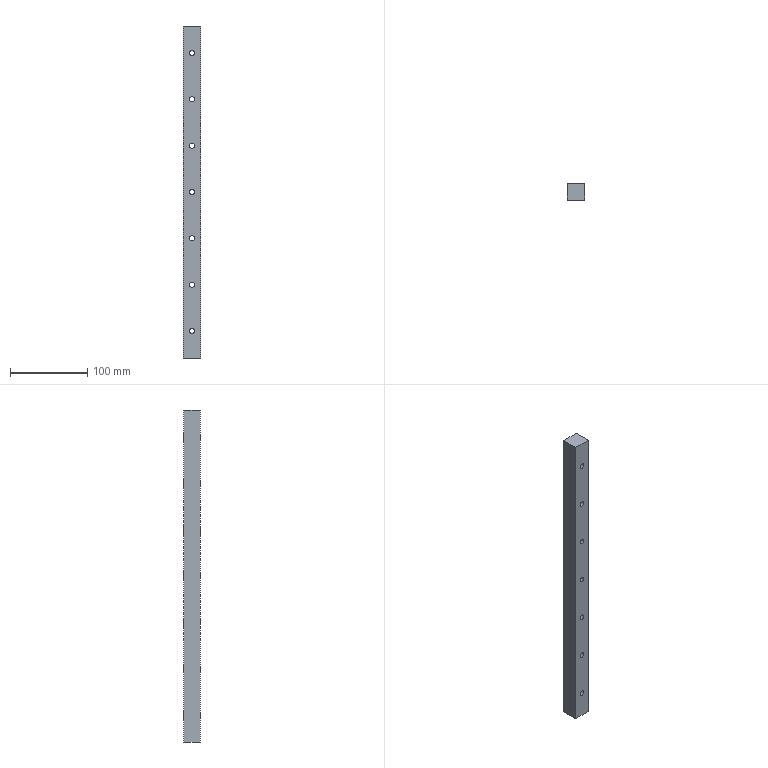Part | SolidWorks | features Extrusion 1, HoleWzd 1, LPattern 1 | 1 solid | 41 faces | box 23 x 22 x 430 mm | volume 209587 mm3 | cylinder 28 | plane 13 | commonest cylinder face diameters 6.6 x14 11 x14
STEP:
#1=CARTESIAN_POINT('',(11.5,0.,31.7));
#2=VERTEX_POINT('',#1);
#3=CARTESIAN_POINT('',(11.5,0.,38.3));
#4=VERTEX_POINT('',#3);
#5=CARTESIAN_POINT('',(11.5,0.,35.));
#6=DIRECTION('',(0.,1.,0.));
#7=DIRECTION('',(0.,0.,1.));
#8=AXIS2_PLACEMENT_3D('',#5,#6,#7);
#9=CIRCLE('',#8,3.3);
#10=EDGE_CURVE('',#2,#4,#9,.T.);
#11=ORIENTED_EDGE('',*,*,#10,.F.);
#12=CARTESIAN_POINT('',(11.5,15.6,31.7));
#13=VERTEX_POINT('',#12);
#14=CARTESIAN_POINT('',(11.5,22.,31.7));
#15=DIRECTION('',(0.,1.,0.));
#16=VECTOR('',#15,1000.);
#17=LINE('',#14,#16);
#18=EDGE_CURVE('',#2,#13,#17,.T.);
#19=ORIENTED_EDGE('',*,*,#18,.T.);
#20=CARTESIAN_POINT('',(11.5,15.6,38.3));
#21=VERTEX_POINT('',#20);
#22=CARTESIAN_POINT('',(11.5,15.6,35.));
#23=DIRECTION('',(0.,1.,0.));
#24=DIRECTION('',(0.,0.,1.));
#25=AXIS2_PLACEMENT_3D('',#22,#23,#24);
#26=CIRCLE('',#25,3.3);
#27=EDGE_CURVE('',#13,#21,#26,.T.);
#28=ORIENTED_EDGE('',*,*,#27,.T.);
#29=CARTESIAN_POINT('',(11.5,22.,38.3));
#30=DIRECTION('',(0.,1.,0.));
#31=VECTOR('',#30,1000.);
#32=LINE('',#29,#31);
#33=EDGE_CURVE('',#4,#21,#32,.T.);
#34=ORIENTED_EDGE('',*,*,#33,.F.);
#35=EDGE_LOOP('',(#11,#19,#28,#34));
#36=FACE_OUTER_BOUND('',#35,.T.);
#37=CARTESIAN_POINT('',(11.5,22.,35.));
#38=DIRECTION('',(0.,1.,0.));
#39=DIRECTION('',(0.,0.,1.));
#40=AXIS2_PLACEMENT_3D('',#37,#38,#39);
#41=CYLINDRICAL_SURFACE('',#40,3.3);
#42=ADVANCED_FACE('',(#36),#41,.F.);
#43=CARTESIAN_POINT('',(11.5,15.6,29.5));
#44=VERTEX_POINT('',#43);
#45=CARTESIAN_POINT('',(11.5,15.6,40.5));
#46=VERTEX_POINT('',#45);
#47=CARTESIAN_POINT('',(11.5,15.6,35.));
#48=DIRECTION('',(0.,1.,0.));
#49=DIRECTION('',(0.,0.,1.));
#50=AXIS2_PLACEMENT_3D('',#47,#48,#49);
#51=CIRCLE('',#50,5.5);
#52=EDGE_CURVE('',#44,#46,#51,.T.);
#53=ORIENTED_EDGE('',*,*,#52,.F.);
#54=CARTESIAN_POINT('',(11.5,22.,29.5));
#55=VERTEX_POINT('',#54);
#56=CARTESIAN_POINT('',(11.5,22.,29.5));
#57=DIRECTION('',(0.,1.,0.));
#58=VECTOR('',#57,1000.);
#59=LINE('',#56,#58);
#60=EDGE_CURVE('',#44,#55,#59,.T.);
#61=ORIENTED_EDGE('',*,*,#60,.T.);
#62=CARTESIAN_POINT('',(11.5,22.,40.5));
#63=VERTEX_POINT('',#62);
#64=CARTESIAN_POINT('',(11.5,22.,35.));
#65=DIRECTION('',(0.,1.,0.));
#66=DIRECTION('',(0.,0.,1.));
#67=AXIS2_PLACEMENT_3D('',#64,#65,#66);
#68=CIRCLE('',#67,5.5);
#69=EDGE_CURVE('',#55,#63,#68,.T.);
#70=ORIENTED_EDGE('',*,*,#69,.T.);
#71=CARTESIAN_POINT('',(11.5,22.,40.5));
#72=DIRECTION('',(0.,1.,0.));
#73=VECTOR('',#72,1000.);
#74=LINE('',#71,#73);
#75=EDGE_CURVE('',#46,#63,#74,.T.);
#76=ORIENTED_EDGE('',*,*,#75,.F.);
#77=EDGE_LOOP('',(#53,#61,#70,#76));
#78=FACE_OUTER_BOUND('',#77,.T.);
#79=CARTESIAN_POINT('',(11.5,22.,35.));
#80=DIRECTION('',(0.,1.,0.));
#81=DIRECTION('',(0.,0.,1.));
#82=AXIS2_PLACEMENT_3D('',#79,#80,#81);
#83=CYLINDRICAL_SURFACE('',#82,5.5);
#84=ADVANCED_FACE('',(#78),#83,.F.);
#85=CARTESIAN_POINT('',(11.5,0.,91.7));
#86=VERTEX_POINT('',#85);
#87=CARTESIAN_POINT('',(11.5,0.,98.3));
#88=VERTEX_POINT('',#87);
#89=CARTESIAN_POINT('',(11.5,0.,95.));
#90=DIRECTION('',(0.,1.,0.));
#91=DIRECTION('',(0.,0.,1.));
#92=AXIS2_PLACEMENT_3D('',#89,#90,#91);
#93=CIRCLE('',#92,3.3);
#94=EDGE_CURVE('',#86,#88,#93,.T.);
#95=ORIENTED_EDGE('',*,*,#94,.F.);
#96=CARTESIAN_POINT('',(11.5,15.6,91.7));
#97=VERTEX_POINT('',#96);
#98=CARTESIAN_POINT('',(11.5,22.,91.7));
#99=DIRECTION('',(0.,1.,0.));
#100=VECTOR('',#99,1000.);
#101=LINE('',#98,#100);
#102=EDGE_CURVE('',#86,#97,#101,.T.);
#103=ORIENTED_EDGE('',*,*,#102,.T.);
#104=CARTESIAN_POINT('',(11.5,15.6,98.3));
#105=VERTEX_POINT('',#104);
#106=CARTESIAN_POINT('',(11.5,15.6,95.));
#107=DIRECTION('',(0.,1.,0.));
#108=DIRECTION('',(0.,0.,1.));
#109=AXIS2_PLACEMENT_3D('',#106,#107,#108);
#110=CIRCLE('',#109,3.3);
#111=EDGE_CURVE('',#97,#105,#110,.T.);
#112=ORIENTED_EDGE('',*,*,#111,.T.);
#113=CARTESIAN_POINT('',(11.5,22.,98.3));
#114=DIRECTION('',(0.,1.,0.));
#115=VECTOR('',#114,1000.);
#116=LINE('',#113,#115);
#117=EDGE_CURVE('',#88,#105,#116,.T.);
#118=ORIENTED_EDGE('',*,*,#117,.F.);
#119=EDGE_LOOP('',(#95,#103,#112,#118));
#120=FACE_OUTER_BOUND('',#119,.T.);
#121=CARTESIAN_POINT('',(11.5,22.,95.));
#122=DIRECTION('',(0.,1.,0.));
#123=DIRECTION('',(0.,0.,1.));
#124=AXIS2_PLACEMENT_3D('',#121,#122,#123);
#125=CYLINDRICAL_SURFACE('',#124,3.3);
#126=ADVANCED_FACE('',(#120),#125,.F.);
#127=CARTESIAN_POINT('',(11.5,15.6,89.5));
#128=VERTEX_POINT('',#127);
#129=CARTESIAN_POINT('',(11.5,15.6,100.5));
#130=VERTEX_POINT('',#129);
#131=CARTESIAN_POINT('',(11.5,15.6,95.));
#132=DIRECTION('',(0.,1.,0.));
#133=DIRECTION('',(0.,0.,1.));
#134=AXIS2_PLACEMENT_3D('',#131,#132,#133);
#135=CIRCLE('',#134,5.5);
#136=EDGE_CURVE('',#128,#130,#135,.T.);
#137=ORIENTED_EDGE('',*,*,#136,.F.);
#138=CARTESIAN_POINT('',(11.5,22.,89.5));
#139=VERTEX_POINT('',#138);
#140=CARTESIAN_POINT('',(11.5,22.,89.5));
#141=DIRECTION('',(0.,1.,0.));
#142=VECTOR('',#141,1000.);
#143=LINE('',#140,#142);
#144=EDGE_CURVE('',#128,#139,#143,.T.);
#145=ORIENTED_EDGE('',*,*,#144,.T.);
#146=CARTESIAN_POINT('',(11.5,22.,100.5));
#147=VERTEX_POINT('',#146);
#148=CARTESIAN_POINT('',(11.5,22.,95.));
#149=DIRECTION('',(0.,1.,0.));
#150=DIRECTION('',(0.,0.,1.));
#151=AXIS2_PLACEMENT_3D('',#148,#149,#150);
#152=CIRCLE('',#151,5.5);
#153=EDGE_CURVE('',#139,#147,#152,.T.);
#154=ORIENTED_EDGE('',*,*,#153,.T.);
#155=CARTESIAN_POINT('',(11.5,22.,100.5));
#156=DIRECTION('',(0.,1.,0.));
#157=VECTOR('',#156,1000.);
#158=LINE('',#155,#157);
#159=EDGE_CURVE('',#130,#147,#158,.T.);
#160=ORIENTED_EDGE('',*,*,#159,.F.);
#161=EDGE_LOOP('',(#137,#145,#154,#160));
#162=FACE_OUTER_BOUND('',#161,.T.);
#163=CARTESIAN_POINT('',(11.5,22.,95.));
#164=DIRECTION('',(0.,1.,0.));
#165=DIRECTION('',(0.,0.,1.));
#166=AXIS2_PLACEMENT_3D('',#163,#164,#165);
#167=CYLINDRICAL_SURFACE('',#166,5.5);
#168=ADVANCED_FACE('',(#162),#167,.F.);
#169=CARTESIAN_POINT('',(11.5,0.,151.7));
#170=VERTEX_POINT('',#169);
#171=CARTESIAN_POINT('',(11.5,0.,158.3));
#172=VERTEX_POINT('',#171);
#173=CARTESIAN_POINT('',(11.5,0.,155.));
#174=DIRECTION('',(0.,1.,0.));
#175=DIRECTION('',(0.,0.,1.));
#176=AXIS2_PLACEMENT_3D('',#173,#174,#175);
#177=CIRCLE('',#176,3.3);
#178=EDGE_CURVE('',#170,#172,#177,.T.);
#179=ORIENTED_EDGE('',*,*,#178,.F.);
#180=CARTESIAN_POINT('',(11.5,15.6,151.7));
#181=VERTEX_POINT('',#180);
#182=CARTESIAN_POINT('',(11.5,22.,151.7));
#183=DIRECTION('',(0.,1.,0.));
#184=VECTOR('',#183,1000.);
#185=LINE('',#182,#184);
#186=EDGE_CURVE('',#170,#181,#185,.T.);
#187=ORIENTED_EDGE('',*,*,#186,.T.);
#188=CARTESIAN_POINT('',(11.5,15.6,158.3));
#189=VERTEX_POINT('',#188);
#190=CARTESIAN_POINT('',(11.5,15.6,155.));
#191=DIRECTION('',(0.,1.,0.));
#192=DIRECTION('',(0.,0.,1.));
#193=AXIS2_PLACEMENT_3D('',#190,#191,#192);
#194=CIRCLE('',#193,3.3);
#195=EDGE_CURVE('',#181,#189,#194,.T.);
#196=ORIENTED_EDGE('',*,*,#195,.T.);
#197=CARTESIAN_POINT('',(11.5,22.,158.3));
#198=DIRECTION('',(0.,1.,0.));
#199=VECTOR('',#198,1000.);
#200=LINE('',#197,#199);
#201=EDGE_CURVE('',#172,#189,#200,.T.);
#202=ORIENTED_EDGE('',*,*,#201,.F.);
#203=EDGE_LOOP('',(#179,#187,#196,#202));
#204=FACE_OUTER_BOUND('',#203,.T.);
#205=CARTESIAN_POINT('',(11.5,22.,155.));
#206=DIRECTION('',(0.,1.,0.));
#207=DIRECTION('',(0.,0.,1.));
#208=AXIS2_PLACEMENT_3D('',#205,#206,#207);
#209=CYLINDRICAL_SURFACE('',#208,3.3);
#210=ADVANCED_FACE('',(#204),#209,.F.);
#211=CARTESIAN_POINT('',(11.5,15.6,149.5));
#212=VERTEX_POINT('',#211);
#213=CARTESIAN_POINT('',(11.5,15.6,160.5));
#214=VERTEX_POINT('',#213);
#215=CARTESIAN_POINT('',(11.5,15.6,155.));
#216=DIRECTION('',(0.,1.,0.));
#217=DIRECTION('',(0.,0.,1.));
#218=AXIS2_PLACEMENT_3D('',#215,#216,#217);
#219=CIRCLE('',#218,5.5);
#220=EDGE_CURVE('',#212,#214,#219,.T.);
#221=ORIENTED_EDGE('',*,*,#220,.F.);
#222=CARTESIAN_POINT('',(11.5,22.,149.5));
#223=VERTEX_POINT('',#222);
#224=CARTESIAN_POINT('',(11.5,22.,149.5));
#225=DIRECTION('',(0.,1.,0.));
#226=VECTOR('',#225,1000.);
#227=LINE('',#224,#226);
#228=EDGE_CURVE('',#212,#223,#227,.T.);
#229=ORIENTED_EDGE('',*,*,#228,.T.);
#230=CARTESIAN_POINT('',(11.5,22.,160.5));
#231=VERTEX_POINT('',#230);
#232=CARTESIAN_POINT('',(11.5,22.,155.));
#233=DIRECTION('',(0.,1.,0.));
#234=DIRECTION('',(0.,0.,1.));
#235=AXIS2_PLACEMENT_3D('',#232,#233,#234);
#236=CIRCLE('',#235,5.5);
#237=EDGE_CURVE('',#223,#231,#236,.T.);
#238=ORIENTED_EDGE('',*,*,#237,.T.);
#239=CARTESIAN_POINT('',(11.5,22.,160.5));
#240=DIRECTION('',(0.,1.,0.));
#241=VECTOR('',#240,1000.);
#242=LINE('',#239,#241);
#243=EDGE_CURVE('',#214,#231,#242,.T.);
#244=ORIENTED_EDGE('',*,*,#243,.F.);
#245=EDGE_LOOP('',(#221,#229,#238,#244));
#246=FACE_OUTER_BOUND('',#245,.T.);
#247=CARTESIAN_POINT('',(11.5,22.,155.));
#248=DIRECTION('',(0.,1.,0.));
#249=DIRECTION('',(0.,0.,1.));
#250=AXIS2_PLACEMENT_3D('',#247,#248,#249);
#251=CYLINDRICAL_SURFACE('',#250,5.5);
#252=ADVANCED_FACE('',(#246),#251,.F.);
#253=CARTESIAN_POINT('',(11.5,0.,211.7));
#254=VERTEX_POINT('',#253);
#255=CARTESIAN_POINT('',(11.5,0.,218.3));
#256=VERTEX_POINT('',#255);
#257=CARTESIAN_POINT('',(11.5,0.,215.));
#258=DIRECTION('',(0.,1.,0.));
#259=DIRECTION('',(0.,0.,1.));
#260=AXIS2_PLACEMENT_3D('',#257,#258,#259);
#261=CIRCLE('',#260,3.3);
#262=EDGE_CURVE('',#254,#256,#261,.T.);
#263=ORIENTED_EDGE('',*,*,#262,.F.);
#264=CARTESIAN_POINT('',(11.5,15.6,211.7));
#265=VERTEX_POINT('',#264);
#266=CARTESIAN_POINT('',(11.5,22.,211.7));
#267=DIRECTION('',(0.,1.,0.));
#268=VECTOR('',#267,1000.);
#269=LINE('',#266,#268);
#270=EDGE_CURVE('',#254,#265,#269,.T.);
#271=ORIENTED_EDGE('',*,*,#270,.T.);
#272=CARTESIAN_POINT('',(11.5,15.6,218.3));
#273=VERTEX_POINT('',#272);
#274=CARTESIAN_POINT('',(11.5,15.6,215.));
#275=DIRECTION('',(0.,1.,0.));
#276=DIRECTION('',(0.,0.,1.));
#277=AXIS2_PLACEMENT_3D('',#274,#275,#276);
#278=CIRCLE('',#277,3.3);
#279=EDGE_CURVE('',#265,#273,#278,.T.);
#280=ORIENTED_EDGE('',*,*,#279,.T.);
#281=CARTESIAN_POINT('',(11.5,22.,218.3));
#282=DIRECTION('',(0.,1.,0.));
#283=VECTOR('',#282,1000.);
#284=LINE('',#281,#283);
#285=EDGE_CURVE('',#256,#273,#284,.T.);
#286=ORIENTED_EDGE('',*,*,#285,.F.);
#287=EDGE_LOOP('',(#263,#271,#280,#286));
#288=FACE_OUTER_BOUND('',#287,.T.);
#289=CARTESIAN_POINT('',(11.5,22.,215.));
#290=DIRECTION('',(0.,1.,0.));
#291=DIRECTION('',(0.,0.,1.));
#292=AXIS2_PLACEMENT_3D('',#289,#290,#291);
#293=CYLINDRICAL_SURFACE('',#292,3.3);
#294=ADVANCED_FACE('',(#288),#293,.F.);
#295=CARTESIAN_POINT('',(11.5,15.6,209.5));
#296=VERTEX_POINT('',#295);
#297=CARTESIAN_POINT('',(11.5,15.6,220.5));
#298=VERTEX_POINT('',#297);
#299=CARTESIAN_POINT('',(11.5,15.6,215.));
#300=DIRECTION('',(0.,1.,0.));
#301=DIRECTION('',(0.,0.,1.));
#302=AXIS2_PLACEMENT_3D('',#299,#300,#301);
#303=CIRCLE('',#302,5.5);
#304=EDGE_CURVE('',#296,#298,#303,.T.);
#305=ORIENTED_EDGE('',*,*,#304,.F.);
#306=CARTESIAN_POINT('',(11.5,22.,209.5));
#307=VERTEX_POINT('',#306);
#308=CARTESIAN_POINT('',(11.5,22.,209.5));
#309=DIRECTION('',(0.,1.,0.));
#310=VECTOR('',#309,1000.);
#311=LINE('',#308,#310);
#312=EDGE_CURVE('',#296,#307,#311,.T.);
#313=ORIENTED_EDGE('',*,*,#312,.T.);
#314=CARTESIAN_POINT('',(11.5,22.,220.5));
#315=VERTEX_POINT('',#314);
#316=CARTESIAN_POINT('',(11.5,22.,215.));
#317=DIRECTION('',(0.,1.,0.));
#318=DIRECTION('',(0.,0.,1.));
#319=AXIS2_PLACEMENT_3D('',#316,#317,#318);
#320=CIRCLE('',#319,5.5);
#321=EDGE_CURVE('',#307,#315,#320,.T.);
#322=ORIENTED_EDGE('',*,*,#321,.T.);
#323=CARTESIAN_POINT('',(11.5,22.,220.5));
#324=DIRECTION('',(0.,1.,0.));
#325=VECTOR('',#324,1000.);
#326=LINE('',#323,#325);
#327=EDGE_CURVE('',#298,#315,#326,.T.);
#328=ORIENTED_EDGE('',*,*,#327,.F.);
#329=EDGE_LOOP('',(#305,#313,#322,#328));
#330=FACE_OUTER_BOUND('',#329,.T.);
#331=CARTESIAN_POINT('',(11.5,22.,215.));
#332=DIRECTION('',(0.,1.,0.));
#333=DIRECTION('',(0.,0.,1.));
#334=AXIS2_PLACEMENT_3D('',#331,#332,#333);
#335=CYLINDRICAL_SURFACE('',#334,5.5);
#336=ADVANCED_FACE('',(#330),#335,.F.);
#337=CARTESIAN_POINT('',(11.5,0.,271.7));
#338=VERTEX_POINT('',#337);
#339=CARTESIAN_POINT('',(11.5,0.,278.3));
#340=VERTEX_POINT('',#339);
#341=CARTESIAN_POINT('',(11.5,0.,275.));
#342=DIRECTION('',(0.,1.,0.));
#343=DIRECTION('',(0.,0.,1.));
#344=AXIS2_PLACEMENT_3D('',#341,#342,#343);
#345=CIRCLE('',#344,3.3);
#346=EDGE_CURVE('',#338,#340,#345,.T.);
#347=ORIENTED_EDGE('',*,*,#346,.F.);
#348=CARTESIAN_POINT('',(11.5,15.6,271.7));
#349=VERTEX_POINT('',#348);
#350=CARTESIAN_POINT('',(11.5,22.,271.7));
#351=DIRECTION('',(0.,1.,0.));
#352=VECTOR('',#351,1000.);
#353=LINE('',#350,#352);
#354=EDGE_CURVE('',#338,#349,#353,.T.);
#355=ORIENTED_EDGE('',*,*,#354,.T.);
#356=CARTESIAN_POINT('',(11.5,15.6,278.3));
#357=VERTEX_POINT('',#356);
#358=CARTESIAN_POINT('',(11.5,15.6,275.));
#359=DIRECTION('',(0.,1.,0.));
#360=DIRECTION('',(0.,0.,1.));
#361=AXIS2_PLACEMENT_3D('',#358,#359,#360);
#362=CIRCLE('',#361,3.3);
#363=EDGE_CURVE('',#349,#357,#362,.T.);
#364=ORIENTED_EDGE('',*,*,#363,.T.);
#365=CARTESIAN_POINT('',(11.5,22.,278.3));
#366=DIRECTION('',(0.,1.,0.));
#367=VECTOR('',#366,1000.);
#368=LINE('',#365,#367);
#369=EDGE_CURVE('',#340,#357,#368,.T.);
#370=ORIENTED_EDGE('',*,*,#369,.F.);
#371=EDGE_LOOP('',(#347,#355,#364,#370));
#372=FACE_OUTER_BOUND('',#371,.T.);
#373=CARTESIAN_POINT('',(11.5,22.,275.));
#374=DIRECTION('',(0.,1.,0.));
#375=DIRECTION('',(0.,0.,1.));
#376=AXIS2_PLACEMENT_3D('',#373,#374,#375);
#377=CYLINDRICAL_SURFACE('',#376,3.3);
#378=ADVANCED_FACE('',(#372),#377,.F.);
#379=CARTESIAN_POINT('',(11.5,15.6,269.5));
#380=VERTEX_POINT('',#379);
#381=CARTESIAN_POINT('',(11.5,15.6,280.5));
#382=VERTEX_POINT('',#381);
#383=CARTESIAN_POINT('',(11.5,15.6,275.));
#384=DIRECTION('',(0.,1.,0.));
#385=DIRECTION('',(0.,0.,1.));
#386=AXIS2_PLACEMENT_3D('',#383,#384,#385);
#387=CIRCLE('',#386,5.5);
#388=EDGE_CURVE('',#380,#382,#387,.T.);
#389=ORIENTED_EDGE('',*,*,#388,.F.);
#390=CARTESIAN_POINT('',(11.5,22.,269.5));
#391=VERTEX_POINT('',#390);
#392=CARTESIAN_POINT('',(11.5,22.,269.5));
#393=DIRECTION('',(0.,1.,0.));
#394=VECTOR('',#393,1000.);
#395=LINE('',#392,#394);
#396=EDGE_CURVE('',#380,#391,#395,.T.);
#397=ORIENTED_EDGE('',*,*,#396,.T.);
#398=CARTESIAN_POINT('',(11.5,22.,280.5));
#399=VERTEX_POINT('',#398);
#400=CARTESIAN_POINT('',(11.5,22.,275.));
#401=DIRECTION('',(0.,1.,0.));
#402=DIRECTION('',(0.,0.,1.));
#403=AXIS2_PLACEMENT_3D('',#400,#401,#402);
#404=CIRCLE('',#403,5.5);
#405=EDGE_CURVE('',#391,#399,#404,.T.);
#406=ORIENTED_EDGE('',*,*,#405,.T.);
#407=CARTESIAN_POINT('',(11.5,22.,280.5));
#408=DIRECTION('',(0.,1.,0.));
#409=VECTOR('',#408,1000.);
#410=LINE('',#407,#409);
#411=EDGE_CURVE('',#382,#399,#410,.T.);
#412=ORIENTED_EDGE('',*,*,#411,.F.);
#413=EDGE_LOOP('',(#389,#397,#406,#412));
#414=FACE_OUTER_BOUND('',#413,.T.);
#415=CARTESIAN_POINT('',(11.5,22.,275.));
#416=DIRECTION('',(0.,1.,0.));
#417=DIRECTION('',(0.,0.,1.));
#418=AXIS2_PLACEMENT_3D('',#415,#416,#417);
#419=CYLINDRICAL_SURFACE('',#418,5.5);
#420=ADVANCED_FACE('',(#414),#419,.F.);
#421=CARTESIAN_POINT('',(11.5,15.6,329.5));
#422=VERTEX_POINT('',#421);
#423=CARTESIAN_POINT('',(11.5,15.6,340.5));
#424=VERTEX_POINT('',#423);
#425=CARTESIAN_POINT('',(11.5,15.6,335.));
#426=DIRECTION('',(0.,1.,0.));
#427=DIRECTION('',(0.,0.,1.));
#428=AXIS2_PLACEMENT_3D('',#425,#426,#427);
#429=CIRCLE('',#428,5.5);
#430=EDGE_CURVE('',#422,#424,#429,.T.);
#431=ORIENTED_EDGE('',*,*,#430,.F.);
#432=CARTESIAN_POINT('',(11.5,22.,329.5));
#433=VERTEX_POINT('',#432);
#434=CARTESIAN_POINT('',(11.5,22.,329.5));
#435=DIRECTION('',(0.,1.,0.));
#436=VECTOR('',#435,1000.);
#437=LINE('',#434,#436);
#438=EDGE_CURVE('',#422,#433,#437,.T.);
#439=ORIENTED_EDGE('',*,*,#438,.T.);
#440=CARTESIAN_POINT('',(11.5,22.,340.5));
#441=VERTEX_POINT('',#440);
#442=CARTESIAN_POINT('',(11.5,22.,335.));
#443=DIRECTION('',(0.,1.,0.));
#444=DIRECTION('',(0.,0.,1.));
#445=AXIS2_PLACEMENT_3D('',#442,#443,#444);
#446=CIRCLE('',#445,5.5);
#447=EDGE_CURVE('',#433,#441,#446,.T.);
#448=ORIENTED_EDGE('',*,*,#447,.T.);
#449=CARTESIAN_POINT('',(11.5,22.,340.5));
#450=DIRECTION('',(0.,1.,0.));
#451=VECTOR('',#450,1000.);
#452=LINE('',#449,#451);
#453=EDGE_CURVE('',#424,#441,#452,.T.);
#454=ORIENTED_EDGE('',*,*,#453,.F.);
#455=EDGE_LOOP('',(#431,#439,#448,#454));
#456=FACE_OUTER_BOUND('',#455,.T.);
#457=CARTESIAN_POINT('',(11.5,22.,335.));
#458=DIRECTION('',(0.,1.,0.));
#459=DIRECTION('',(0.,0.,1.));
#460=AXIS2_PLACEMENT_3D('',#457,#458,#459);
#461=CYLINDRICAL_SURFACE('',#460,5.5);
#462=ADVANCED_FACE('',(#456),#461,.F.);
#463=CARTESIAN_POINT('',(11.5,0.,331.7));
#464=VERTEX_POINT('',#463);
#465=CARTESIAN_POINT('',(11.5,0.,338.3));
#466=VERTEX_POINT('',#465);
#467=CARTESIAN_POINT('',(11.5,0.,335.));
#468=DIRECTION('',(0.,1.,0.));
#469=DIRECTION('',(0.,0.,1.));
#470=AXIS2_PLACEMENT_3D('',#467,#468,#469);
#471=CIRCLE('',#470,3.3);
#472=EDGE_CURVE('',#464,#466,#471,.T.);
#473=ORIENTED_EDGE('',*,*,#472,.F.);
#474=CARTESIAN_POINT('',(11.5,15.6,331.7));
#475=VERTEX_POINT('',#474);
#476=CARTESIAN_POINT('',(11.5,22.,331.7));
#477=DIRECTION('',(0.,1.,0.));
#478=VECTOR('',#477,1000.);
#479=LINE('',#476,#478);
#480=EDGE_CURVE('',#464,#475,#479,.T.);
#481=ORIENTED_EDGE('',*,*,#480,.T.);
#482=CARTESIAN_POINT('',(11.5,15.6,338.3));
#483=VERTEX_POINT('',#482);
#484=CARTESIAN_POINT('',(11.5,15.6,335.));
#485=DIRECTION('',(0.,1.,0.));
#486=DIRECTION('',(0.,0.,1.));
#487=AXIS2_PLACEMENT_3D('',#484,#485,#486);
#488=CIRCLE('',#487,3.3);
#489=EDGE_CURVE('',#475,#483,#488,.T.);
#490=ORIENTED_EDGE('',*,*,#489,.T.);
#491=CARTESIAN_POINT('',(11.5,22.,338.3));
#492=DIRECTION('',(0.,1.,0.));
#493=VECTOR('',#492,1000.);
#494=LINE('',#491,#493);
#495=EDGE_CURVE('',#466,#483,#494,.T.);
#496=ORIENTED_EDGE('',*,*,#495,.F.);
#497=EDGE_LOOP('',(#473,#481,#490,#496));
#498=FACE_OUTER_BOUND('',#497,.T.);
#499=CARTESIAN_POINT('',(11.5,22.,335.));
#500=DIRECTION('',(0.,1.,0.));
#501=DIRECTION('',(0.,0.,1.));
#502=AXIS2_PLACEMENT_3D('',#499,#500,#501);
#503=CYLINDRICAL_SURFACE('',#502,3.3);
#504=ADVANCED_FACE('',(#498),#503,.F.);
#505=CARTESIAN_POINT('',(11.5,15.6,389.5));
#506=VERTEX_POINT('',#505);
#507=CARTESIAN_POINT('',(11.5,15.6,400.5));
#508=VERTEX_POINT('',#507);
#509=CARTESIAN_POINT('',(11.5,15.6,395.));
#510=DIRECTION('',(0.,1.,0.));
#511=DIRECTION('',(0.,0.,1.));
#512=AXIS2_PLACEMENT_3D('',#509,#510,#511);
#513=CIRCLE('',#512,5.5);
#514=EDGE_CURVE('',#506,#508,#513,.T.);
#515=ORIENTED_EDGE('',*,*,#514,.F.);
#516=CARTESIAN_POINT('',(11.5,22.,389.5));
#517=VERTEX_POINT('',#516);
#518=CARTESIAN_POINT('',(11.5,22.,389.5));
#519=DIRECTION('',(0.,1.,0.));
#520=VECTOR('',#519,1000.);
#521=LINE('',#518,#520);
#522=EDGE_CURVE('',#506,#517,#521,.T.);
#523=ORIENTED_EDGE('',*,*,#522,.T.);
#524=CARTESIAN_POINT('',(11.5,22.,400.5));
#525=VERTEX_POINT('',#524);
#526=CARTESIAN_POINT('',(11.5,22.,395.));
#527=DIRECTION('',(0.,1.,0.));
#528=DIRECTION('',(0.,0.,1.));
#529=AXIS2_PLACEMENT_3D('',#526,#527,#528);
#530=CIRCLE('',#529,5.5);
#531=EDGE_CURVE('',#517,#525,#530,.T.);
#532=ORIENTED_EDGE('',*,*,#531,.T.);
#533=CARTESIAN_POINT('',(11.5,22.,400.5));
#534=DIRECTION('',(0.,1.,0.));
#535=VECTOR('',#534,1000.);
#536=LINE('',#533,#535);
#537=EDGE_CURVE('',#508,#525,#536,.T.);
#538=ORIENTED_EDGE('',*,*,#537,.F.);
#539=EDGE_LOOP('',(#515,#523,#532,#538));
#540=FACE_OUTER_BOUND('',#539,.T.);
#541=CARTESIAN_POINT('',(11.5,22.,395.));
#542=DIRECTION('',(0.,1.,0.));
#543=DIRECTION('',(0.,0.,1.));
#544=AXIS2_PLACEMENT_3D('',#541,#542,#543);
#545=CYLINDRICAL_SURFACE('',#544,5.5);
#546=ADVANCED_FACE('',(#540),#545,.F.);
#547=CARTESIAN_POINT('',(11.5,0.,391.7));
#548=VERTEX_POINT('',#547);
#549=CARTESIAN_POINT('',(11.5,0.,398.3));
#550=VERTEX_POINT('',#549);
#551=CARTESIAN_POINT('',(11.5,0.,395.));
#552=DIRECTION('',(0.,1.,0.));
#553=DIRECTION('',(0.,0.,1.));
#554=AXIS2_PLACEMENT_3D('',#551,#552,#553);
#555=CIRCLE('',#554,3.3);
#556=EDGE_CURVE('',#548,#550,#555,.T.);
#557=ORIENTED_EDGE('',*,*,#556,.F.);
#558=CARTESIAN_POINT('',(11.5,15.6,391.7));
#559=VERTEX_POINT('',#558);
#560=CARTESIAN_POINT('',(11.5,22.,391.7));
#561=DIRECTION('',(0.,1.,0.));
#562=VECTOR('',#561,1000.);
#563=LINE('',#560,#562);
#564=EDGE_CURVE('',#548,#559,#563,.T.);
#565=ORIENTED_EDGE('',*,*,#564,.T.);
#566=CARTESIAN_POINT('',(11.5,15.6,398.3));
#567=VERTEX_POINT('',#566);
#568=CARTESIAN_POINT('',(11.5,15.6,395.));
#569=DIRECTION('',(0.,1.,0.));
#570=DIRECTION('',(0.,0.,1.));
#571=AXIS2_PLACEMENT_3D('',#568,#569,#570);
#572=CIRCLE('',#571,3.3);
#573=EDGE_CURVE('',#559,#567,#572,.T.);
#574=ORIENTED_EDGE('',*,*,#573,.T.);
#575=CARTESIAN_POINT('',(11.5,22.,398.3));
#576=DIRECTION('',(0.,1.,0.));
#577=VECTOR('',#576,1000.);
#578=LINE('',#575,#577);
#579=EDGE_CURVE('',#550,#567,#578,.T.);
#580=ORIENTED_EDGE('',*,*,#579,.F.);
#581=EDGE_LOOP('',(#557,#565,#574,#580));
#582=FACE_OUTER_BOUND('',#581,.T.);
#583=CARTESIAN_POINT('',(11.5,22.,395.));
#584=DIRECTION('',(0.,1.,0.));
#585=DIRECTION('',(0.,0.,1.));
#586=AXIS2_PLACEMENT_3D('',#583,#584,#585);
#587=CYLINDRICAL_SURFACE('',#586,3.3);
#588=ADVANCED_FACE('',(#582),#587,.F.);
#589=CARTESIAN_POINT('',(0.,22.,0.));
#590=VERTEX_POINT('',#589);
#591=CARTESIAN_POINT('',(0.,0.,0.));
#592=VERTEX_POINT('',#591);
#593=CARTESIAN_POINT('',(0.,0.,0.));
#594=DIRECTION('',(0.,-1.,0.));
#595=VECTOR('',#594,1000.);
#596=LINE('',#593,#595);
#597=EDGE_CURVE('',#590,#592,#596,.T.);
#598=ORIENTED_EDGE('',*,*,#597,.T.);
#599=CARTESIAN_POINT('',(0.,0.,430.));
#600=VERTEX_POINT('',#599);
#601=CARTESIAN_POINT('',(0.,0.,430.));
#602=DIRECTION('',(0.,0.,-1.));
#603=VECTOR('',#602,1000.);
#604=LINE('',#601,#603);
#605=EDGE_CURVE('',#600,#592,#604,.T.);
#606=ORIENTED_EDGE('',*,*,#605,.F.);
#607=CARTESIAN_POINT('',(0.,22.,430.));
#608=VERTEX_POINT('',#607);
#609=CARTESIAN_POINT('',(0.,0.,430.));
#610=DIRECTION('',(0.,-1.,0.));
#611=VECTOR('',#610,1000.);
#612=LINE('',#609,#611);
#613=EDGE_CURVE('',#608,#600,#612,.T.);
#614=ORIENTED_EDGE('',*,*,#613,.F.);
#615=CARTESIAN_POINT('',(0.,22.,430.));
#616=DIRECTION('',(0.,0.,-1.));
#617=VECTOR('',#616,1000.);
#618=LINE('',#615,#617);
#619=EDGE_CURVE('',#608,#590,#618,.T.);
#620=ORIENTED_EDGE('',*,*,#619,.T.);
#621=EDGE_LOOP('',(#598,#606,#614,#620));
#622=FACE_OUTER_BOUND('',#621,.T.);
#623=CARTESIAN_POINT('',(0.,0.,430.));
#624=DIRECTION('',(1.,0.,0.));
#625=DIRECTION('',(0.,1.,0.));
#626=AXIS2_PLACEMENT_3D('',#623,#624,#625);
#627=PLANE('',#626);
#628=ADVANCED_FACE('',(#622),#627,.F.);
#629=CARTESIAN_POINT('',(11.5,0.,335.));
#630=DIRECTION('',(0.,1.,0.));
#631=DIRECTION('',(0.,0.,1.));
#632=AXIS2_PLACEMENT_3D('',#629,#630,#631);
#633=CIRCLE('',#632,3.3);
#634=EDGE_CURVE('',#466,#464,#633,.T.);
#635=ORIENTED_EDGE('',*,*,#634,.T.);
#636=ORIENTED_EDGE('',*,*,#472,.T.);
#637=EDGE_LOOP('',(#635,#636));
#638=FACE_BOUND('',#637,.T.);
#639=CARTESIAN_POINT('',(11.5,0.,395.));
#640=DIRECTION('',(0.,1.,0.));
#641=DIRECTION('',(0.,0.,1.));
#642=AXIS2_PLACEMENT_3D('',#639,#640,#641);
#643=CIRCLE('',#642,3.3);
#644=EDGE_CURVE('',#550,#548,#643,.T.);
#645=ORIENTED_EDGE('',*,*,#644,.T.);
#646=ORIENTED_EDGE('',*,*,#556,.T.);
#647=EDGE_LOOP('',(#645,#646));
#648=FACE_BOUND('',#647,.T.);
#649=CARTESIAN_POINT('',(23.,0.,0.));
#650=VERTEX_POINT('',#649);
#651=CARTESIAN_POINT('',(0.,0.,0.));
#652=DIRECTION('',(1.,0.,0.));
#653=VECTOR('',#652,1000.);
#654=LINE('',#651,#653);
#655=EDGE_CURVE('',#592,#650,#654,.T.);
#656=ORIENTED_EDGE('',*,*,#655,.T.);
#657=CARTESIAN_POINT('',(23.,0.,430.));
#658=VERTEX_POINT('',#657);
#659=CARTESIAN_POINT('',(23.,0.,430.));
#660=DIRECTION('',(0.,0.,-1.));
#661=VECTOR('',#660,1000.);
#662=LINE('',#659,#661);
#663=EDGE_CURVE('',#658,#650,#662,.T.);
#664=ORIENTED_EDGE('',*,*,#663,.F.);
#665=CARTESIAN_POINT('',(0.,0.,430.));
#666=DIRECTION('',(1.,0.,0.));
#667=VECTOR('',#666,1000.);
#668=LINE('',#665,#667);
#669=EDGE_CURVE('',#600,#658,#668,.T.);
#670=ORIENTED_EDGE('',*,*,#669,.F.);
#671=ORIENTED_EDGE('',*,*,#605,.T.);
#672=EDGE_LOOP('',(#656,#664,#670,#671));
#673=FACE_OUTER_BOUND('',#672,.T.);
#674=CARTESIAN_POINT('',(11.5,0.,275.));
#675=DIRECTION('',(0.,1.,0.));
#676=DIRECTION('',(0.,0.,1.));
#677=AXIS2_PLACEMENT_3D('',#674,#675,#676);
#678=CIRCLE('',#677,3.3);
#679=EDGE_CURVE('',#340,#338,#678,.T.);
#680=ORIENTED_EDGE('',*,*,#679,.T.);
#681=ORIENTED_EDGE('',*,*,#346,.T.);
#682=EDGE_LOOP('',(#680,#681));
#683=FACE_BOUND('',#682,.T.);
#684=CARTESIAN_POINT('',(11.5,0.,215.));
#685=DIRECTION('',(0.,1.,0.));
#686=DIRECTION('',(0.,0.,1.));
#687=AXIS2_PLACEMENT_3D('',#684,#685,#686);
#688=CIRCLE('',#687,3.3);
#689=EDGE_CURVE('',#256,#254,#688,.T.);
#690=ORIENTED_EDGE('',*,*,#689,.T.);
#691=ORIENTED_EDGE('',*,*,#262,.T.);
#692=EDGE_LOOP('',(#690,#691));
#693=FACE_BOUND('',#692,.T.);
#694=CARTESIAN_POINT('',(11.5,0.,155.));
#695=DIRECTION('',(0.,1.,0.));
#696=DIRECTION('',(0.,0.,1.));
#697=AXIS2_PLACEMENT_3D('',#694,#695,#696);
#698=CIRCLE('',#697,3.3);
#699=EDGE_CURVE('',#172,#170,#698,.T.);
#700=ORIENTED_EDGE('',*,*,#699,.T.);
#701=ORIENTED_EDGE('',*,*,#178,.T.);
#702=EDGE_LOOP('',(#700,#701));
#703=FACE_BOUND('',#702,.T.);
#704=CARTESIAN_POINT('',(11.5,0.,95.));
#705=DIRECTION('',(0.,1.,0.));
#706=DIRECTION('',(0.,0.,1.));
#707=AXIS2_PLACEMENT_3D('',#704,#705,#706);
#708=CIRCLE('',#707,3.3);
#709=EDGE_CURVE('',#88,#86,#708,.T.);
#710=ORIENTED_EDGE('',*,*,#709,.T.);
#711=ORIENTED_EDGE('',*,*,#94,.T.);
#712=EDGE_LOOP('',(#710,#711));
#713=FACE_BOUND('',#712,.T.);
#714=CARTESIAN_POINT('',(11.5,0.,35.));
#715=DIRECTION('',(0.,1.,0.));
#716=DIRECTION('',(0.,0.,1.));
#717=AXIS2_PLACEMENT_3D('',#714,#715,#716);
#718=CIRCLE('',#717,3.3);
#719=EDGE_CURVE('',#4,#2,#718,.T.);
#720=ORIENTED_EDGE('',*,*,#719,.T.);
#721=ORIENTED_EDGE('',*,*,#10,.T.);
#722=EDGE_LOOP('',(#720,#721));
#723=FACE_BOUND('',#722,.T.);
#724=CARTESIAN_POINT('',(0.,0.,430.));
#725=DIRECTION('',(0.,1.,0.));
#726=DIRECTION('',(0.,0.,1.));
#727=AXIS2_PLACEMENT_3D('',#724,#725,#726);
#728=PLANE('',#727);
#729=ADVANCED_FACE('',(#638,#648,#673,#683,#693,#703,#713,#723),#728,.F.);
#730=CARTESIAN_POINT('',(23.,22.,0.));
#731=VERTEX_POINT('',#730);
#732=CARTESIAN_POINT('',(23.,0.,0.));
#733=DIRECTION('',(0.,1.,0.));
#734=VECTOR('',#733,1000.);
#735=LINE('',#732,#734);
#736=EDGE_CURVE('',#650,#731,#735,.T.);
#737=ORIENTED_EDGE('',*,*,#736,.T.);
#738=CARTESIAN_POINT('',(23.,22.,430.));
#739=VERTEX_POINT('',#738);
#740=CARTESIAN_POINT('',(23.,22.,430.));
#741=DIRECTION('',(0.,0.,-1.));
#742=VECTOR('',#741,1000.);
#743=LINE('',#740,#742);
#744=EDGE_CURVE('',#739,#731,#743,.T.);
#745=ORIENTED_EDGE('',*,*,#744,.F.);
#746=CARTESIAN_POINT('',(23.,0.,430.));
#747=DIRECTION('',(0.,1.,0.));
#748=VECTOR('',#747,1000.);
#749=LINE('',#746,#748);
#750=EDGE_CURVE('',#658,#739,#749,.T.);
#751=ORIENTED_EDGE('',*,*,#750,.F.);
#752=ORIENTED_EDGE('',*,*,#663,.T.);
#753=EDGE_LOOP('',(#737,#745,#751,#752));
#754=FACE_OUTER_BOUND('',#753,.T.);
#755=CARTESIAN_POINT('',(23.,0.,430.));
#756=DIRECTION('',(-1.,0.,0.));
#757=DIRECTION('',(0.,-1.,0.));
#758=AXIS2_PLACEMENT_3D('',#755,#756,#757);
#759=PLANE('',#758);
#760=ADVANCED_FACE('',(#754),#759,.F.);
#761=CARTESIAN_POINT('',(11.5,22.,335.));
#762=DIRECTION('',(0.,1.,0.));
#763=DIRECTION('',(0.,0.,1.));
#764=AXIS2_PLACEMENT_3D('',#761,#762,#763);
#765=CIRCLE('',#764,5.5);
#766=EDGE_CURVE('',#441,#433,#765,.T.);
#767=ORIENTED_EDGE('',*,*,#766,.F.);
#768=ORIENTED_EDGE('',*,*,#447,.F.);
#769=EDGE_LOOP('',(#767,#768));
#770=FACE_BOUND('',#769,.T.);
#771=CARTESIAN_POINT('',(11.5,22.,395.));
#772=DIRECTION('',(0.,1.,0.));
#773=DIRECTION('',(0.,0.,1.));
#774=AXIS2_PLACEMENT_3D('',#771,#772,#773);
#775=CIRCLE('',#774,5.5);
#776=EDGE_CURVE('',#525,#517,#775,.T.);
#777=ORIENTED_EDGE('',*,*,#776,.F.);
#778=ORIENTED_EDGE('',*,*,#531,.F.);
#779=EDGE_LOOP('',(#777,#778));
#780=FACE_BOUND('',#779,.T.);
#781=CARTESIAN_POINT('',(0.,22.,0.));
#782=DIRECTION('',(-1.,0.,0.));
#783=VECTOR('',#782,1000.);
#784=LINE('',#781,#783);
#785=EDGE_CURVE('',#731,#590,#784,.T.);
#786=ORIENTED_EDGE('',*,*,#785,.T.);
#787=ORIENTED_EDGE('',*,*,#619,.F.);
#788=CARTESIAN_POINT('',(0.,22.,430.));
#789=DIRECTION('',(-1.,0.,0.));
#790=VECTOR('',#789,1000.);
#791=LINE('',#788,#790);
#792=EDGE_CURVE('',#739,#608,#791,.T.);
#793=ORIENTED_EDGE('',*,*,#792,.F.);
#794=ORIENTED_EDGE('',*,*,#744,.T.);
#795=EDGE_LOOP('',(#786,#787,#793,#794));
#796=FACE_OUTER_BOUND('',#795,.T.);
#797=CARTESIAN_POINT('',(11.5,22.,275.));
#798=DIRECTION('',(0.,1.,0.));
#799=DIRECTION('',(0.,0.,1.));
#800=AXIS2_PLACEMENT_3D('',#797,#798,#799);
#801=CIRCLE('',#800,5.5);
#802=EDGE_CURVE('',#399,#391,#801,.T.);
#803=ORIENTED_EDGE('',*,*,#802,.F.);
#804=ORIENTED_EDGE('',*,*,#405,.F.);
#805=EDGE_LOOP('',(#803,#804));
#806=FACE_BOUND('',#805,.T.);
#807=CARTESIAN_POINT('',(11.5,22.,215.));
#808=DIRECTION('',(0.,1.,0.));
#809=DIRECTION('',(0.,0.,1.));
#810=AXIS2_PLACEMENT_3D('',#807,#808,#809);
#811=CIRCLE('',#810,5.5);
#812=EDGE_CURVE('',#315,#307,#811,.T.);
#813=ORIENTED_EDGE('',*,*,#812,.F.);
#814=ORIENTED_EDGE('',*,*,#321,.F.);
#815=EDGE_LOOP('',(#813,#814));
#816=FACE_BOUND('',#815,.T.);
#817=CARTESIAN_POINT('',(11.5,22.,155.));
#818=DIRECTION('',(0.,1.,0.));
#819=DIRECTION('',(0.,0.,1.));
#820=AXIS2_PLACEMENT_3D('',#817,#818,#819);
#821=CIRCLE('',#820,5.5);
#822=EDGE_CURVE('',#231,#223,#821,.T.);
#823=ORIENTED_EDGE('',*,*,#822,.F.);
#824=ORIENTED_EDGE('',*,*,#237,.F.);
#825=EDGE_LOOP('',(#823,#824));
#826=FACE_BOUND('',#825,.T.);
#827=CARTESIAN_POINT('',(11.5,22.,95.));
#828=DIRECTION('',(0.,1.,0.));
#829=DIRECTION('',(0.,0.,1.));
#830=AXIS2_PLACEMENT_3D('',#827,#828,#829);
#831=CIRCLE('',#830,5.5);
#832=EDGE_CURVE('',#147,#139,#831,.T.);
#833=ORIENTED_EDGE('',*,*,#832,.F.);
#834=ORIENTED_EDGE('',*,*,#153,.F.);
#835=EDGE_LOOP('',(#833,#834));
#836=FACE_BOUND('',#835,.T.);
#837=CARTESIAN_POINT('',(11.5,22.,35.));
#838=DIRECTION('',(0.,1.,0.));
#839=DIRECTION('',(0.,0.,1.));
#840=AXIS2_PLACEMENT_3D('',#837,#838,#839);
#841=CIRCLE('',#840,5.5);
#842=EDGE_CURVE('',#63,#55,#841,.T.);
#843=ORIENTED_EDGE('',*,*,#842,.F.);
#844=ORIENTED_EDGE('',*,*,#69,.F.);
#845=EDGE_LOOP('',(#843,#844));
#846=FACE_BOUND('',#845,.T.);
#847=CARTESIAN_POINT('',(0.,22.,430.));
#848=DIRECTION('',(0.,-1.,0.));
#849=DIRECTION('',(0.,0.,-1.));
#850=AXIS2_PLACEMENT_3D('',#847,#848,#849);
#851=PLANE('',#850);
#852=ADVANCED_FACE('',(#770,#780,#796,#806,#816,#826,#836,#846),#851,.F.);
#853=ORIENTED_EDGE('',*,*,#613,.T.);
#854=ORIENTED_EDGE('',*,*,#669,.T.);
#855=ORIENTED_EDGE('',*,*,#750,.T.);
#856=ORIENTED_EDGE('',*,*,#792,.T.);
#857=EDGE_LOOP('',(#853,#854,#855,#856));
#858=FACE_OUTER_BOUND('',#857,.T.);
#859=CARTESIAN_POINT('',(0.,0.,430.));
#860=DIRECTION('',(0.,0.,-1.));
#861=DIRECTION('',(-1.,0.,0.));
#862=AXIS2_PLACEMENT_3D('',#859,#860,#861);
#863=PLANE('',#862);
#864=ADVANCED_FACE('',(#858),#863,.F.);
#865=ORIENTED_EDGE('',*,*,#597,.F.);
#866=ORIENTED_EDGE('',*,*,#785,.F.);
#867=ORIENTED_EDGE('',*,*,#736,.F.);
#868=ORIENTED_EDGE('',*,*,#655,.F.);
#869=EDGE_LOOP('',(#865,#866,#867,#868));
#870=FACE_OUTER_BOUND('',#869,.T.);
#871=CARTESIAN_POINT('',(0.,0.,0.));
#872=DIRECTION('',(0.,0.,-1.));
#873=DIRECTION('',(-1.,0.,0.));
#874=AXIS2_PLACEMENT_3D('',#871,#872,#873);
#875=PLANE('',#874);
#876=ADVANCED_FACE('',(#870),#875,.T.);
#877=ORIENTED_EDGE('',*,*,#564,.F.);
#878=ORIENTED_EDGE('',*,*,#644,.F.);
#879=ORIENTED_EDGE('',*,*,#579,.T.);
#880=CARTESIAN_POINT('',(11.5,15.6,395.));
#881=DIRECTION('',(0.,1.,0.));
#882=DIRECTION('',(0.,0.,1.));
#883=AXIS2_PLACEMENT_3D('',#880,#881,#882);
#884=CIRCLE('',#883,3.3);
#885=EDGE_CURVE('',#567,#559,#884,.T.);
#886=ORIENTED_EDGE('',*,*,#885,.T.);
#887=EDGE_LOOP('',(#877,#878,#879,#886));
#888=FACE_OUTER_BOUND('',#887,.T.);
#889=CARTESIAN_POINT('',(11.5,22.,395.));
#890=DIRECTION('',(0.,1.,0.));
#891=DIRECTION('',(0.,0.,1.));
#892=AXIS2_PLACEMENT_3D('',#889,#890,#891);
#893=CYLINDRICAL_SURFACE('',#892,3.3);
#894=ADVANCED_FACE('',(#888),#893,.F.);
#895=ORIENTED_EDGE('',*,*,#885,.F.);
#896=ORIENTED_EDGE('',*,*,#573,.F.);
#897=EDGE_LOOP('',(#895,#896));
#898=FACE_BOUND('',#897,.T.);
#899=CARTESIAN_POINT('',(11.5,15.6,395.));
#900=DIRECTION('',(0.,1.,0.));
#901=DIRECTION('',(0.,0.,1.));
#902=AXIS2_PLACEMENT_3D('',#899,#900,#901);
#903=CIRCLE('',#902,5.5);
#904=EDGE_CURVE('',#508,#506,#903,.T.);
#905=ORIENTED_EDGE('',*,*,#904,.T.);
#906=ORIENTED_EDGE('',*,*,#514,.T.);
#907=EDGE_LOOP('',(#905,#906));
#908=FACE_OUTER_BOUND('',#907,.T.);
#909=CARTESIAN_POINT('',(14.8,15.6,395.));
#910=DIRECTION('',(0.,-1.,0.));
#911=DIRECTION('',(0.,0.,-1.));
#912=AXIS2_PLACEMENT_3D('',#909,#910,#911);
#913=PLANE('',#912);
#914=ADVANCED_FACE('',(#898,#908),#913,.F.);
#915=ORIENTED_EDGE('',*,*,#522,.F.);
#916=ORIENTED_EDGE('',*,*,#904,.F.);
#917=ORIENTED_EDGE('',*,*,#537,.T.);
#918=ORIENTED_EDGE('',*,*,#776,.T.);
#919=EDGE_LOOP('',(#915,#916,#917,#918));
#920=FACE_OUTER_BOUND('',#919,.T.);
#921=CARTESIAN_POINT('',(11.5,22.,395.));
#922=DIRECTION('',(0.,1.,0.));
#923=DIRECTION('',(0.,0.,1.));
#924=AXIS2_PLACEMENT_3D('',#921,#922,#923);
#925=CYLINDRICAL_SURFACE('',#924,5.5);
#926=ADVANCED_FACE('',(#920),#925,.F.);
#927=ORIENTED_EDGE('',*,*,#480,.F.);
#928=ORIENTED_EDGE('',*,*,#634,.F.);
#929=ORIENTED_EDGE('',*,*,#495,.T.);
#930=CARTESIAN_POINT('',(11.5,15.6,335.));
#931=DIRECTION('',(0.,1.,0.));
#932=DIRECTION('',(0.,0.,1.));
#933=AXIS2_PLACEMENT_3D('',#930,#931,#932);
#934=CIRCLE('',#933,3.3);
#935=EDGE_CURVE('',#483,#475,#934,.T.);
#936=ORIENTED_EDGE('',*,*,#935,.T.);
#937=EDGE_LOOP('',(#927,#928,#929,#936));
#938=FACE_OUTER_BOUND('',#937,.T.);
#939=CARTESIAN_POINT('',(11.5,22.,335.));
#940=DIRECTION('',(0.,1.,0.));
#941=DIRECTION('',(0.,0.,1.));
#942=AXIS2_PLACEMENT_3D('',#939,#940,#941);
#943=CYLINDRICAL_SURFACE('',#942,3.3);
#944=ADVANCED_FACE('',(#938),#943,.F.);
#945=ORIENTED_EDGE('',*,*,#935,.F.);
#946=ORIENTED_EDGE('',*,*,#489,.F.);
#947=EDGE_LOOP('',(#945,#946));
#948=FACE_BOUND('',#947,.T.);
#949=CARTESIAN_POINT('',(11.5,15.6,335.));
#950=DIRECTION('',(0.,1.,0.));
#951=DIRECTION('',(0.,0.,1.));
#952=AXIS2_PLACEMENT_3D('',#949,#950,#951);
#953=CIRCLE('',#952,5.5);
#954=EDGE_CURVE('',#424,#422,#953,.T.);
#955=ORIENTED_EDGE('',*,*,#954,.T.);
#956=ORIENTED_EDGE('',*,*,#430,.T.);
#957=EDGE_LOOP('',(#955,#956));
#958=FACE_OUTER_BOUND('',#957,.T.);
#959=CARTESIAN_POINT('',(14.8,15.6,335.));
#960=DIRECTION('',(0.,-1.,0.));
#961=DIRECTION('',(0.,0.,-1.));
#962=AXIS2_PLACEMENT_3D('',#959,#960,#961);
#963=PLANE('',#962);
#964=ADVANCED_FACE('',(#948,#958),#963,.F.);
#965=ORIENTED_EDGE('',*,*,#438,.F.);
#966=ORIENTED_EDGE('',*,*,#954,.F.);
#967=ORIENTED_EDGE('',*,*,#453,.T.);
#968=ORIENTED_EDGE('',*,*,#766,.T.);
#969=EDGE_LOOP('',(#965,#966,#967,#968));
#970=FACE_OUTER_BOUND('',#969,.T.);
#971=CARTESIAN_POINT('',(11.5,22.,335.));
#972=DIRECTION('',(0.,1.,0.));
#973=DIRECTION('',(0.,0.,1.));
#974=AXIS2_PLACEMENT_3D('',#971,#972,#973);
#975=CYLINDRICAL_SURFACE('',#974,5.5);
#976=ADVANCED_FACE('',(#970),#975,.F.);
#977=ORIENTED_EDGE('',*,*,#396,.F.);
#978=CARTESIAN_POINT('',(11.5,15.6,275.));
#979=DIRECTION('',(0.,1.,0.));
#980=DIRECTION('',(0.,0.,1.));
#981=AXIS2_PLACEMENT_3D('',#978,#979,#980);
#982=CIRCLE('',#981,5.5);
#983=EDGE_CURVE('',#382,#380,#982,.T.);
#984=ORIENTED_EDGE('',*,*,#983,.F.);
#985=ORIENTED_EDGE('',*,*,#411,.T.);
#986=ORIENTED_EDGE('',*,*,#802,.T.);
#987=EDGE_LOOP('',(#977,#984,#985,#986));
#988=FACE_OUTER_BOUND('',#987,.T.);
#989=CARTESIAN_POINT('',(11.5,22.,275.));
#990=DIRECTION('',(0.,1.,0.));
#991=DIRECTION('',(0.,0.,1.));
#992=AXIS2_PLACEMENT_3D('',#989,#990,#991);
#993=CYLINDRICAL_SURFACE('',#992,5.5);
#994=ADVANCED_FACE('',(#988),#993,.F.);
#995=CARTESIAN_POINT('',(11.5,15.6,275.));
#996=DIRECTION('',(0.,1.,0.));
#997=DIRECTION('',(0.,0.,1.));
#998=AXIS2_PLACEMENT_3D('',#995,#996,#997);
#999=CIRCLE('',#998,3.3);
#1000=EDGE_CURVE('',#357,#349,#999,.T.);
#1001=ORIENTED_EDGE('',*,*,#1000,.F.);
#1002=ORIENTED_EDGE('',*,*,#363,.F.);
#1003=EDGE_LOOP('',(#1001,#1002));
#1004=FACE_BOUND('',#1003,.T.);
#1005=ORIENTED_EDGE('',*,*,#983,.T.);
#1006=ORIENTED_EDGE('',*,*,#388,.T.);
#1007=EDGE_LOOP('',(#1005,#1006));
#1008=FACE_OUTER_BOUND('',#1007,.T.);
#1009=CARTESIAN_POINT('',(14.8,15.6,275.));
#1010=DIRECTION('',(0.,-1.,0.));
#1011=DIRECTION('',(0.,0.,-1.));
#1012=AXIS2_PLACEMENT_3D('',#1009,#1010,#1011);
#1013=PLANE('',#1012);
#1014=ADVANCED_FACE('',(#1004,#1008),#1013,.F.);
#1015=ORIENTED_EDGE('',*,*,#354,.F.);
#1016=ORIENTED_EDGE('',*,*,#679,.F.);
#1017=ORIENTED_EDGE('',*,*,#369,.T.);
#1018=ORIENTED_EDGE('',*,*,#1000,.T.);
#1019=EDGE_LOOP('',(#1015,#1016,#1017,#1018));
#1020=FACE_OUTER_BOUND('',#1019,.T.);
#1021=CARTESIAN_POINT('',(11.5,22.,275.));
#1022=DIRECTION('',(0.,1.,0.));
#1023=DIRECTION('',(0.,0.,1.));
#1024=AXIS2_PLACEMENT_3D('',#1021,#1022,#1023);
#1025=CYLINDRICAL_SURFACE('',#1024,3.3);
#1026=ADVANCED_FACE('',(#1020),#1025,.F.);
#1027=ORIENTED_EDGE('',*,*,#312,.F.);
#1028=CARTESIAN_POINT('',(11.5,15.6,215.));
#1029=DIRECTION('',(0.,1.,0.));
#1030=DIRECTION('',(0.,0.,1.));
#1031=AXIS2_PLACEMENT_3D('',#1028,#1029,#1030);
#1032=CIRCLE('',#1031,5.5);
#1033=EDGE_CURVE('',#298,#296,#1032,.T.);
#1034=ORIENTED_EDGE('',*,*,#1033,.F.);
#1035=ORIENTED_EDGE('',*,*,#327,.T.);
#1036=ORIENTED_EDGE('',*,*,#812,.T.);
#1037=EDGE_LOOP('',(#1027,#1034,#1035,#1036));
#1038=FACE_OUTER_BOUND('',#1037,.T.);
#1039=CARTESIAN_POINT('',(11.5,22.,215.));
#1040=DIRECTION('',(0.,1.,0.));
#1041=DIRECTION('',(0.,0.,1.));
#1042=AXIS2_PLACEMENT_3D('',#1039,#1040,#1041);
#1043=CYLINDRICAL_SURFACE('',#1042,5.5);
#1044=ADVANCED_FACE('',(#1038),#1043,.F.);
#1045=CARTESIAN_POINT('',(11.5,15.6,215.));
#1046=DIRECTION('',(0.,1.,0.));
#1047=DIRECTION('',(0.,0.,1.));
#1048=AXIS2_PLACEMENT_3D('',#1045,#1046,#1047);
#1049=CIRCLE('',#1048,3.3);
#1050=EDGE_CURVE('',#273,#265,#1049,.T.);
#1051=ORIENTED_EDGE('',*,*,#1050,.F.);
#1052=ORIENTED_EDGE('',*,*,#279,.F.);
#1053=EDGE_LOOP('',(#1051,#1052));
#1054=FACE_BOUND('',#1053,.T.);
#1055=ORIENTED_EDGE('',*,*,#1033,.T.);
#1056=ORIENTED_EDGE('',*,*,#304,.T.);
#1057=EDGE_LOOP('',(#1055,#1056));
#1058=FACE_OUTER_BOUND('',#1057,.T.);
#1059=CARTESIAN_POINT('',(14.8,15.6,215.));
#1060=DIRECTION('',(0.,-1.,0.));
#1061=DIRECTION('',(0.,0.,-1.));
#1062=AXIS2_PLACEMENT_3D('',#1059,#1060,#1061);
#1063=PLANE('',#1062);
#1064=ADVANCED_FACE('',(#1054,#1058),#1063,.F.);
#1065=ORIENTED_EDGE('',*,*,#270,.F.);
#1066=ORIENTED_EDGE('',*,*,#689,.F.);
#1067=ORIENTED_EDGE('',*,*,#285,.T.);
#1068=ORIENTED_EDGE('',*,*,#1050,.T.);
#1069=EDGE_LOOP('',(#1065,#1066,#1067,#1068));
#1070=FACE_OUTER_BOUND('',#1069,.T.);
#1071=CARTESIAN_POINT('',(11.5,22.,215.));
#1072=DIRECTION('',(0.,1.,0.));
#1073=DIRECTION('',(0.,0.,1.));
#1074=AXIS2_PLACEMENT_3D('',#1071,#1072,#1073);
#1075=CYLINDRICAL_SURFACE('',#1074,3.3);
#1076=ADVANCED_FACE('',(#1070),#1075,.F.);
#1077=ORIENTED_EDGE('',*,*,#228,.F.);
#1078=CARTESIAN_POINT('',(11.5,15.6,155.));
#1079=DIRECTION('',(0.,1.,0.));
#1080=DIRECTION('',(0.,0.,1.));
#1081=AXIS2_PLACEMENT_3D('',#1078,#1079,#1080);
#1082=CIRCLE('',#1081,5.5);
#1083=EDGE_CURVE('',#214,#212,#1082,.T.);
#1084=ORIENTED_EDGE('',*,*,#1083,.F.);
#1085=ORIENTED_EDGE('',*,*,#243,.T.);
#1086=ORIENTED_EDGE('',*,*,#822,.T.);
#1087=EDGE_LOOP('',(#1077,#1084,#1085,#1086));
#1088=FACE_OUTER_BOUND('',#1087,.T.);
#1089=CARTESIAN_POINT('',(11.5,22.,155.));
#1090=DIRECTION('',(0.,1.,0.));
#1091=DIRECTION('',(0.,0.,1.));
#1092=AXIS2_PLACEMENT_3D('',#1089,#1090,#1091);
#1093=CYLINDRICAL_SURFACE('',#1092,5.5);
#1094=ADVANCED_FACE('',(#1088),#1093,.F.);
#1095=CARTESIAN_POINT('',(11.5,15.6,155.));
#1096=DIRECTION('',(0.,1.,0.));
#1097=DIRECTION('',(0.,0.,1.));
#1098=AXIS2_PLACEMENT_3D('',#1095,#1096,#1097);
#1099=CIRCLE('',#1098,3.3);
#1100=EDGE_CURVE('',#189,#181,#1099,.T.);
#1101=ORIENTED_EDGE('',*,*,#1100,.F.);
#1102=ORIENTED_EDGE('',*,*,#195,.F.);
#1103=EDGE_LOOP('',(#1101,#1102));
#1104=FACE_BOUND('',#1103,.T.);
#1105=ORIENTED_EDGE('',*,*,#1083,.T.);
#1106=ORIENTED_EDGE('',*,*,#220,.T.);
#1107=EDGE_LOOP('',(#1105,#1106));
#1108=FACE_OUTER_BOUND('',#1107,.T.);
#1109=CARTESIAN_POINT('',(14.8,15.6,155.));
#1110=DIRECTION('',(0.,-1.,0.));
#1111=DIRECTION('',(0.,0.,-1.));
#1112=AXIS2_PLACEMENT_3D('',#1109,#1110,#1111);
#1113=PLANE('',#1112);
#1114=ADVANCED_FACE('',(#1104,#1108),#1113,.F.);
#1115=ORIENTED_EDGE('',*,*,#186,.F.);
#1116=ORIENTED_EDGE('',*,*,#699,.F.);
#1117=ORIENTED_EDGE('',*,*,#201,.T.);
#1118=ORIENTED_EDGE('',*,*,#1100,.T.);
#1119=EDGE_LOOP('',(#1115,#1116,#1117,#1118));
#1120=FACE_OUTER_BOUND('',#1119,.T.);
#1121=CARTESIAN_POINT('',(11.5,22.,155.));
#1122=DIRECTION('',(0.,1.,0.));
#1123=DIRECTION('',(0.,0.,1.));
#1124=AXIS2_PLACEMENT_3D('',#1121,#1122,#1123);
#1125=CYLINDRICAL_SURFACE('',#1124,3.3);
#1126=ADVANCED_FACE('',(#1120),#1125,.F.);
#1127=ORIENTED_EDGE('',*,*,#144,.F.);
#1128=CARTESIAN_POINT('',(11.5,15.6,95.));
#1129=DIRECTION('',(0.,1.,0.));
#1130=DIRECTION('',(0.,0.,1.));
#1131=AXIS2_PLACEMENT_3D('',#1128,#1129,#1130);
#1132=CIRCLE('',#1131,5.5);
#1133=EDGE_CURVE('',#130,#128,#1132,.T.);
#1134=ORIENTED_EDGE('',*,*,#1133,.F.);
#1135=ORIENTED_EDGE('',*,*,#159,.T.);
#1136=ORIENTED_EDGE('',*,*,#832,.T.);
#1137=EDGE_LOOP('',(#1127,#1134,#1135,#1136));
#1138=FACE_OUTER_BOUND('',#1137,.T.);
#1139=CARTESIAN_POINT('',(11.5,22.,95.));
#1140=DIRECTION('',(0.,1.,0.));
#1141=DIRECTION('',(0.,0.,1.));
#1142=AXIS2_PLACEMENT_3D('',#1139,#1140,#1141);
#1143=CYLINDRICAL_SURFACE('',#1142,5.5);
#1144=ADVANCED_FACE('',(#1138),#1143,.F.);
#1145=CARTESIAN_POINT('',(11.5,15.6,95.));
#1146=DIRECTION('',(0.,1.,0.));
#1147=DIRECTION('',(0.,0.,1.));
#1148=AXIS2_PLACEMENT_3D('',#1145,#1146,#1147);
#1149=CIRCLE('',#1148,3.3);
#1150=EDGE_CURVE('',#105,#97,#1149,.T.);
#1151=ORIENTED_EDGE('',*,*,#1150,.F.);
#1152=ORIENTED_EDGE('',*,*,#111,.F.);
#1153=EDGE_LOOP('',(#1151,#1152));
#1154=FACE_BOUND('',#1153,.T.);
#1155=ORIENTED_EDGE('',*,*,#1133,.T.);
#1156=ORIENTED_EDGE('',*,*,#136,.T.);
#1157=EDGE_LOOP('',(#1155,#1156));
#1158=FACE_OUTER_BOUND('',#1157,.T.);
#1159=CARTESIAN_POINT('',(14.8,15.6,95.));
#1160=DIRECTION('',(0.,-1.,0.));
#1161=DIRECTION('',(0.,0.,-1.));
#1162=AXIS2_PLACEMENT_3D('',#1159,#1160,#1161);
#1163=PLANE('',#1162);
#1164=ADVANCED_FACE('',(#1154,#1158),#1163,.F.);
#1165=ORIENTED_EDGE('',*,*,#102,.F.);
#1166=ORIENTED_EDGE('',*,*,#709,.F.);
#1167=ORIENTED_EDGE('',*,*,#117,.T.);
#1168=ORIENTED_EDGE('',*,*,#1150,.T.);
#1169=EDGE_LOOP('',(#1165,#1166,#1167,#1168));
#1170=FACE_OUTER_BOUND('',#1169,.T.);
#1171=CARTESIAN_POINT('',(11.5,22.,95.));
#1172=DIRECTION('',(0.,1.,0.));
#1173=DIRECTION('',(0.,0.,1.));
#1174=AXIS2_PLACEMENT_3D('',#1171,#1172,#1173);
#1175=CYLINDRICAL_SURFACE('',#1174,3.3);
#1176=ADVANCED_FACE('',(#1170),#1175,.F.);
#1177=ORIENTED_EDGE('',*,*,#60,.F.);
#1178=CARTESIAN_POINT('',(11.5,15.6,35.));
#1179=DIRECTION('',(0.,1.,0.));
#1180=DIRECTION('',(0.,0.,1.));
#1181=AXIS2_PLACEMENT_3D('',#1178,#1179,#1180);
#1182=CIRCLE('',#1181,5.5);
#1183=EDGE_CURVE('',#46,#44,#1182,.T.);
#1184=ORIENTED_EDGE('',*,*,#1183,.F.);
#1185=ORIENTED_EDGE('',*,*,#75,.T.);
#1186=ORIENTED_EDGE('',*,*,#842,.T.);
#1187=EDGE_LOOP('',(#1177,#1184,#1185,#1186));
#1188=FACE_OUTER_BOUND('',#1187,.T.);
#1189=CARTESIAN_POINT('',(11.5,22.,35.));
#1190=DIRECTION('',(0.,1.,0.));
#1191=DIRECTION('',(0.,0.,1.));
#1192=AXIS2_PLACEMENT_3D('',#1189,#1190,#1191);
#1193=CYLINDRICAL_SURFACE('',#1192,5.5);
#1194=ADVANCED_FACE('',(#1188),#1193,.F.);
#1195=CARTESIAN_POINT('',(11.5,15.6,35.));
#1196=DIRECTION('',(0.,1.,0.));
#1197=DIRECTION('',(0.,0.,1.));
#1198=AXIS2_PLACEMENT_3D('',#1195,#1196,#1197);
#1199=CIRCLE('',#1198,3.3);
#1200=EDGE_CURVE('',#21,#13,#1199,.T.);
#1201=ORIENTED_EDGE('',*,*,#1200,.F.);
#1202=ORIENTED_EDGE('',*,*,#27,.F.);
#1203=EDGE_LOOP('',(#1201,#1202));
#1204=FACE_BOUND('',#1203,.T.);
#1205=ORIENTED_EDGE('',*,*,#1183,.T.);
#1206=ORIENTED_EDGE('',*,*,#52,.T.);
#1207=EDGE_LOOP('',(#1205,#1206));
#1208=FACE_OUTER_BOUND('',#1207,.T.);
#1209=CARTESIAN_POINT('',(14.8,15.6,35.));
#1210=DIRECTION('',(0.,-1.,0.));
#1211=DIRECTION('',(0.,0.,-1.));
#1212=AXIS2_PLACEMENT_3D('',#1209,#1210,#1211);
#1213=PLANE('',#1212);
#1214=ADVANCED_FACE('',(#1204,#1208),#1213,.F.);
#1215=ORIENTED_EDGE('',*,*,#18,.F.);
#1216=ORIENTED_EDGE('',*,*,#719,.F.);
#1217=ORIENTED_EDGE('',*,*,#33,.T.);
#1218=ORIENTED_EDGE('',*,*,#1200,.T.);
#1219=EDGE_LOOP('',(#1215,#1216,#1217,#1218));
#1220=FACE_OUTER_BOUND('',#1219,.T.);
#1221=CARTESIAN_POINT('',(11.5,22.,35.));
#1222=DIRECTION('',(0.,1.,0.));
#1223=DIRECTION('',(0.,0.,1.));
#1224=AXIS2_PLACEMENT_3D('',#1221,#1222,#1223);
#1225=CYLINDRICAL_SURFACE('',#1224,3.3);
#1226=ADVANCED_FACE('',(#1220),#1225,.F.);
#1227=CLOSED_SHELL('',(#42,#84,#126,#168,#210,#252,#294,#336,#378,#420,#462,#504,#546,#588,#628,#729,#760,#852,#864,#876,#894,#914,#926,#944,#964,#976,#994,#1014,#1026,#1044,#1064,#1076,#1094,#1114,#1126,#1144,#1164,#1176,#1194,#1214,#1226));
#1228=MANIFOLD_SOLID_BREP('',#1227);
#1229=CARTESIAN_POINT('',(0.,0.,0.));
#1230=DIRECTION('',(0.,0.,1.));
#1231=DIRECTION('',(1.,0.,0.));
#1232=AXIS2_PLACEMENT_3D('',#1229,#1230,#1231);
#1233=(LENGTH_UNIT()NAMED_UNIT(*)SI_UNIT(.MILLI.,.METRE.));
#1234=UNCERTAINTY_MEASURE_WITH_UNIT(LENGTH_MEASURE(0.00001),#1233,'','');
#1235=(NAMED_UNIT(*)PLANE_ANGLE_UNIT()SI_UNIT($,.RADIAN.));
#1236=(NAMED_UNIT(*)SI_UNIT($,.STERADIAN.)SOLID_ANGLE_UNIT());
#1237=(GEOMETRIC_REPRESENTATION_CONTEXT(3)GLOBAL_UNCERTAINTY_ASSIGNED_CONTEXT((#1234))GLOBAL_UNIT_ASSIGNED_CONTEXT((#1233,#1235,#1236))REPRESENTATION_CONTEXT('',''));
#1238=ADVANCED_BREP_SHAPE_REPRESENTATION('',(#1228,#1232),#1237);